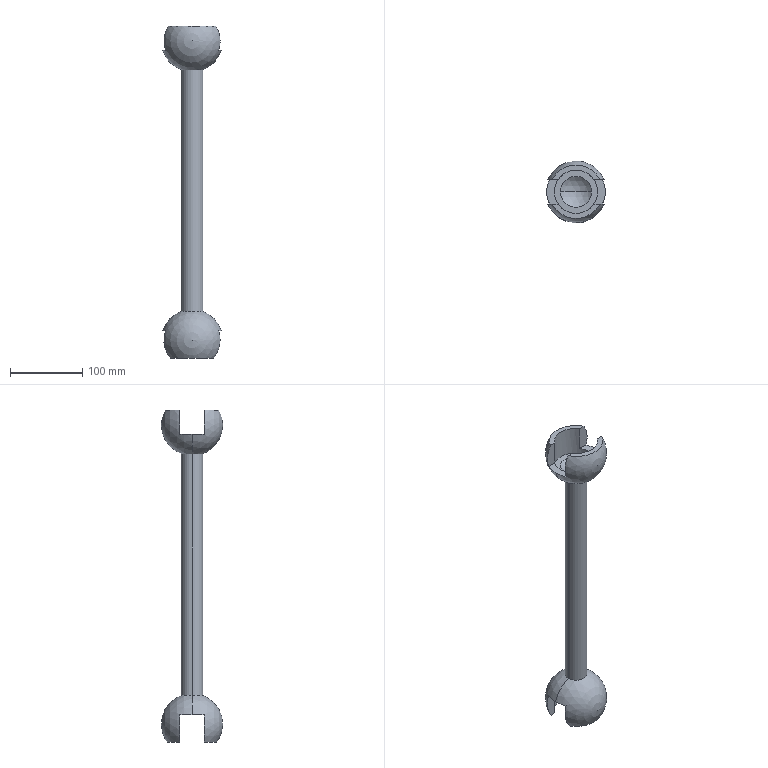Part | SolidWorks | features ICE 3, Chamfer 2, Extrusion 1, MirrorPattern 1, RevCut 1, Revolution 1 | 1 solid | 32 faces | box 80.921 x 85 x 459.451 mm | volume 470589 mm3 | plane 14 | sphere 8 | cylinder 6 | cone 4 | commonest cylinder face diameters 60 x4 30 x2
STEP:
#1=CARTESIAN_POINT('',(0.,0.,279.));
#2=VERTEX_POINT('',#1);
#3=CARTESIAN_POINT('',(-21.424,0.,288.));
#4=VERTEX_POINT('',#3);
#5=CARTESIAN_POINT('',(0.,0.,309.));
#6=DIRECTION('',(0.,1.,0.));
#7=DIRECTION('',(0.,0.,1.));
#8=AXIS2_PLACEMENT_3D('',#5,#6,#7);
#9=CIRCLE('',#8,30.);
#10=EDGE_CURVE('',#2,#4,#9,.T.);
#11=ORIENTED_EDGE('',*,*,#10,.F.);
#12=CARTESIAN_POINT('',(21.424,0.,288.));
#13=VERTEX_POINT('',#12);
#14=CARTESIAN_POINT('',(0.,0.,309.));
#15=DIRECTION('',(0.,-1.,0.));
#16=DIRECTION('',(1.,0.,0.));
#17=AXIS2_PLACEMENT_3D('',#14,#15,#16);
#18=CIRCLE('',#17,30.);
#19=EDGE_CURVE('',#2,#13,#18,.T.);
#20=ORIENTED_EDGE('',*,*,#19,.T.);
#21=CARTESIAN_POINT('',(0.,0.,288.));
#22=DIRECTION('',(0.,0.,1.));
#23=DIRECTION('',(-1.,0.,0.));
#24=AXIS2_PLACEMENT_3D('',#21,#22,#23);
#25=CIRCLE('',#24,21.424);
#26=EDGE_CURVE('',#13,#4,#25,.T.);
#27=ORIENTED_EDGE('',*,*,#26,.T.);
#28=EDGE_LOOP('',(#11,#20,#27));
#29=FACE_OUTER_BOUND('',#28,.T.);
#30=CARTESIAN_POINT('',(0.,0.,309.));
#31=DIRECTION('',(0.,-1.,0.));
#32=DIRECTION('',(-1.,0.,0.));
#33=AXIS2_PLACEMENT_3D('',#30,#31,#32);
#34=SPHERICAL_SURFACE('',#33,30.);
#35=ADVANCED_FACE('',(#29),#34,.F.);
#36=CARTESIAN_POINT('',(-30.,0.,288.));
#37=VERTEX_POINT('',#36);
#38=CARTESIAN_POINT('',(30.,0.,288.));
#39=VERTEX_POINT('',#38);
#40=CARTESIAN_POINT('',(0.,0.,288.));
#41=DIRECTION('',(0.,0.,1.));
#42=DIRECTION('',(1.,0.,0.));
#43=AXIS2_PLACEMENT_3D('',#40,#41,#42);
#44=CIRCLE('',#43,30.);
#45=EDGE_CURVE('',#37,#39,#44,.T.);
#46=ORIENTED_EDGE('',*,*,#45,.F.);
#47=CARTESIAN_POINT('',(-30.,0.,295.992));
#48=VERTEX_POINT('',#47);
#49=CARTESIAN_POINT('',(-30.,0.,288.));
#50=DIRECTION('',(0.,0.,1.));
#51=VECTOR('',#50,1000.);
#52=LINE('',#49,#51);
#53=EDGE_CURVE('',#37,#48,#52,.T.);
#54=ORIENTED_EDGE('',*,*,#53,.T.);
#55=CARTESIAN_POINT('',(-24.577,-17.204,295.992));
#56=VERTEX_POINT('',#55);
#57=CARTESIAN_POINT('',(0.,0.,295.992));
#58=DIRECTION('',(0.,0.,-1.));
#59=DIRECTION('',(1.,0.,0.));
#60=AXIS2_PLACEMENT_3D('',#57,#58,#59);
#61=CIRCLE('',#60,30.);
#62=EDGE_CURVE('',#56,#48,#61,.T.);
#63=ORIENTED_EDGE('',*,*,#62,.F.);
#64=CARTESIAN_POINT('',(-24.577,-17.204,329.749));
#65=VERTEX_POINT('',#64);
#66=CARTESIAN_POINT('',(-24.577,-17.204,288.));
#67=DIRECTION('',(0.,0.,1.));
#68=VECTOR('',#67,1000.);
#69=LINE('',#66,#68);
#70=EDGE_CURVE('',#56,#65,#69,.T.);
#71=ORIENTED_EDGE('',*,*,#70,.T.);
#72=CARTESIAN_POINT('',(24.577,-17.204,329.749));
#73=VERTEX_POINT('',#72);
#74=CARTESIAN_POINT('',(0.,0.,329.749));
#75=DIRECTION('',(0.,0.,1.));
#76=DIRECTION('',(-1.,0.,0.));
#77=AXIS2_PLACEMENT_3D('',#74,#75,#76);
#78=CIRCLE('',#77,30.);
#79=EDGE_CURVE('',#65,#73,#78,.T.);
#80=ORIENTED_EDGE('',*,*,#79,.T.);
#81=CARTESIAN_POINT('',(24.577,-17.204,295.992));
#82=VERTEX_POINT('',#81);
#83=CARTESIAN_POINT('',(24.577,-17.204,288.));
#84=DIRECTION('',(0.,0.,-1.));
#85=VECTOR('',#84,1000.);
#86=LINE('',#83,#85);
#87=EDGE_CURVE('',#73,#82,#86,.T.);
#88=ORIENTED_EDGE('',*,*,#87,.T.);
#89=CARTESIAN_POINT('',(30.,0.,295.992));
#90=VERTEX_POINT('',#89);
#91=CARTESIAN_POINT('',(0.,0.,295.992));
#92=DIRECTION('',(0.,0.,-1.));
#93=DIRECTION('',(1.,0.,0.));
#94=AXIS2_PLACEMENT_3D('',#91,#92,#93);
#95=CIRCLE('',#94,30.);
#96=EDGE_CURVE('',#90,#82,#95,.T.);
#97=ORIENTED_EDGE('',*,*,#96,.F.);
#98=CARTESIAN_POINT('',(30.,0.,288.));
#99=DIRECTION('',(0.,0.,1.));
#100=VECTOR('',#99,1000.);
#101=LINE('',#98,#100);
#102=EDGE_CURVE('',#39,#90,#101,.T.);
#103=ORIENTED_EDGE('',*,*,#102,.F.);
#104=EDGE_LOOP('',(#46,#54,#63,#71,#80,#88,#97,#103));
#105=FACE_OUTER_BOUND('',#104,.T.);
#106=CARTESIAN_POINT('',(0.,0.,288.));
#107=DIRECTION('',(0.,0.,1.));
#108=DIRECTION('',(1.,0.,0.));
#109=AXIS2_PLACEMENT_3D('',#106,#107,#108);
#110=CYLINDRICAL_SURFACE('',#109,30.);
#111=ADVANCED_FACE('',(#105),#110,.F.);
#112=CARTESIAN_POINT('',(15.,0.,269.235));
#113=VERTEX_POINT('',#112);
#114=CARTESIAN_POINT('',(-15.,0.,269.235));
#115=VERTEX_POINT('',#114);
#116=CARTESIAN_POINT('',(0.,0.,269.235));
#117=DIRECTION('',(0.,0.,1.));
#118=DIRECTION('',(1.,0.,0.));
#119=AXIS2_PLACEMENT_3D('',#116,#117,#118);
#120=CIRCLE('',#119,15.);
#121=EDGE_CURVE('',#113,#115,#120,.T.);
#122=ORIENTED_EDGE('',*,*,#121,.T.);
#123=CARTESIAN_POINT('',(-40.46,0.,295.992));
#124=VERTEX_POINT('',#123);
#125=CARTESIAN_POINT('',(0.,0.,309.));
#126=DIRECTION('',(0.,1.,0.));
#127=DIRECTION('',(-1.,0.,0.));
#128=AXIS2_PLACEMENT_3D('',#125,#126,#127);
#129=CIRCLE('',#128,42.5);
#130=EDGE_CURVE('',#115,#124,#129,.T.);
#131=ORIENTED_EDGE('',*,*,#130,.T.);
#132=CARTESIAN_POINT('',(-36.62,17.204,295.992));
#133=VERTEX_POINT('',#132);
#134=CARTESIAN_POINT('',(0.,0.,295.992));
#135=DIRECTION('',(0.,0.,1.));
#136=DIRECTION('',(1.,0.,0.));
#137=AXIS2_PLACEMENT_3D('',#134,#135,#136);
#138=CIRCLE('',#137,40.46);
#139=EDGE_CURVE('',#133,#124,#138,.T.);
#140=ORIENTED_EDGE('',*,*,#139,.F.);
#141=CARTESIAN_POINT('',(-32.854,17.204,329.757));
#142=VERTEX_POINT('',#141);
#143=CARTESIAN_POINT('',(0.,17.204,309.));
#144=DIRECTION('',(0.,-1.,0.));
#145=DIRECTION('',(0.,0.,-1.));
#146=AXIS2_PLACEMENT_3D('',#143,#144,#145);
#147=CIRCLE('',#146,38.862);
#148=EDGE_CURVE('',#142,#133,#147,.T.);
#149=ORIENTED_EDGE('',*,*,#148,.F.);
#150=CARTESIAN_POINT('',(32.854,17.204,329.757));
#151=VERTEX_POINT('',#150);
#152=CARTESIAN_POINT('',(0.,0.,329.757));
#153=DIRECTION('',(0.,0.,-1.));
#154=DIRECTION('',(-1.,0.,0.));
#155=AXIS2_PLACEMENT_3D('',#152,#153,#154);
#156=CIRCLE('',#155,37.086);
#157=EDGE_CURVE('',#142,#151,#156,.T.);
#158=ORIENTED_EDGE('',*,*,#157,.T.);
#159=CARTESIAN_POINT('',(36.62,17.204,295.992));
#160=VERTEX_POINT('',#159);
#161=CARTESIAN_POINT('',(0.,17.204,309.));
#162=DIRECTION('',(0.,-1.,0.));
#163=DIRECTION('',(0.,0.,-1.));
#164=AXIS2_PLACEMENT_3D('',#161,#162,#163);
#165=CIRCLE('',#164,38.862);
#166=EDGE_CURVE('',#160,#151,#165,.T.);
#167=ORIENTED_EDGE('',*,*,#166,.F.);
#168=CARTESIAN_POINT('',(40.46,0.,295.992));
#169=VERTEX_POINT('',#168);
#170=CARTESIAN_POINT('',(0.,0.,295.992));
#171=DIRECTION('',(0.,0.,1.));
#172=DIRECTION('',(1.,0.,0.));
#173=AXIS2_PLACEMENT_3D('',#170,#171,#172);
#174=CIRCLE('',#173,40.46);
#175=EDGE_CURVE('',#169,#160,#174,.T.);
#176=ORIENTED_EDGE('',*,*,#175,.F.);
#177=CARTESIAN_POINT('',(0.,0.,309.));
#178=DIRECTION('',(0.,-1.,0.));
#179=DIRECTION('',(0.,0.,-1.));
#180=AXIS2_PLACEMENT_3D('',#177,#178,#179);
#181=CIRCLE('',#180,42.5);
#182=EDGE_CURVE('',#113,#169,#181,.T.);
#183=ORIENTED_EDGE('',*,*,#182,.F.);
#184=EDGE_LOOP('',(#122,#131,#140,#149,#158,#167,#176,#183));
#185=FACE_OUTER_BOUND('',#184,.T.);
#186=CARTESIAN_POINT('',(0.,0.,309.));
#187=DIRECTION('',(0.,1.,0.));
#188=DIRECTION('',(1.,0.,0.));
#189=AXIS2_PLACEMENT_3D('',#186,#187,#188);
#190=SPHERICAL_SURFACE('',#189,42.5);
#191=ADVANCED_FACE('',(#185),#190,.T.);
#192=CARTESIAN_POINT('',(0.,0.,-75.));
#193=VERTEX_POINT('',#192);
#194=CARTESIAN_POINT('',(-21.424,0.,-84.));
#195=VERTEX_POINT('',#194);
#196=CARTESIAN_POINT('',(0.,0.,-105.));
#197=DIRECTION('',(0.,-1.,0.));
#198=DIRECTION('',(0.,0.,-1.));
#199=AXIS2_PLACEMENT_3D('',#196,#197,#198);
#200=CIRCLE('',#199,30.);
#201=EDGE_CURVE('',#193,#195,#200,.T.);
#202=ORIENTED_EDGE('',*,*,#201,.F.);
#203=CARTESIAN_POINT('',(21.424,0.,-84.));
#204=VERTEX_POINT('',#203);
#205=CARTESIAN_POINT('',(0.,0.,-105.));
#206=DIRECTION('',(0.,1.,0.));
#207=DIRECTION('',(-1.,0.,0.));
#208=AXIS2_PLACEMENT_3D('',#205,#206,#207);
#209=CIRCLE('',#208,30.);
#210=EDGE_CURVE('',#193,#204,#209,.T.);
#211=ORIENTED_EDGE('',*,*,#210,.T.);
#212=CARTESIAN_POINT('',(0.,0.,-84.));
#213=DIRECTION('',(0.,0.,-1.));
#214=DIRECTION('',(1.,0.,0.));
#215=AXIS2_PLACEMENT_3D('',#212,#213,#214);
#216=CIRCLE('',#215,21.424);
#217=EDGE_CURVE('',#204,#195,#216,.T.);
#218=ORIENTED_EDGE('',*,*,#217,.T.);
#219=EDGE_LOOP('',(#202,#211,#218));
#220=FACE_OUTER_BOUND('',#219,.T.);
#221=CARTESIAN_POINT('',(0.,0.,-105.));
#222=DIRECTION('',(0.,1.,0.));
#223=DIRECTION('',(-1.,0.,0.));
#224=AXIS2_PLACEMENT_3D('',#221,#222,#223);
#225=SPHERICAL_SURFACE('',#224,30.);
#226=ADVANCED_FACE('',(#220),#225,.F.);
#227=CARTESIAN_POINT('',(15.,0.,-65.235));
#228=VERTEX_POINT('',#227);
#229=CARTESIAN_POINT('',(-15.,0.,-65.235));
#230=VERTEX_POINT('',#229);
#231=CARTESIAN_POINT('',(0.,0.,-65.235));
#232=DIRECTION('',(0.,0.,-1.));
#233=DIRECTION('',(-1.,0.,0.));
#234=AXIS2_PLACEMENT_3D('',#231,#232,#233);
#235=CIRCLE('',#234,15.);
#236=EDGE_CURVE('',#228,#230,#235,.T.);
#237=ORIENTED_EDGE('',*,*,#236,.T.);
#238=CARTESIAN_POINT('',(-40.46,0.,-91.992));
#239=VERTEX_POINT('',#238);
#240=CARTESIAN_POINT('',(0.,0.,-105.));
#241=DIRECTION('',(0.,-1.,0.));
#242=DIRECTION('',(1.,0.,0.));
#243=AXIS2_PLACEMENT_3D('',#240,#241,#242);
#244=CIRCLE('',#243,42.5);
#245=EDGE_CURVE('',#230,#239,#244,.T.);
#246=ORIENTED_EDGE('',*,*,#245,.T.);
#247=CARTESIAN_POINT('',(-36.62,-17.204,-91.992));
#248=VERTEX_POINT('',#247);
#249=CARTESIAN_POINT('',(0.,0.,-91.992));
#250=DIRECTION('',(0.,0.,1.));
#251=DIRECTION('',(1.,0.,0.));
#252=AXIS2_PLACEMENT_3D('',#249,#250,#251);
#253=CIRCLE('',#252,40.46);
#254=EDGE_CURVE('',#239,#248,#253,.T.);
#255=ORIENTED_EDGE('',*,*,#254,.T.);
#256=CARTESIAN_POINT('',(-30.008,-17.204,-129.694));
#257=VERTEX_POINT('',#256);
#258=CARTESIAN_POINT('',(0.,-17.204,-105.));
#259=DIRECTION('',(0.,1.,0.));
#260=DIRECTION('',(0.,0.,1.));
#261=AXIS2_PLACEMENT_3D('',#258,#259,#260);
#262=CIRCLE('',#261,38.862);
#263=EDGE_CURVE('',#257,#248,#262,.T.);
#264=ORIENTED_EDGE('',*,*,#263,.F.);
#265=CARTESIAN_POINT('',(30.008,-17.204,-129.694));
#266=VERTEX_POINT('',#265);
#267=CARTESIAN_POINT('',(0.,0.,-129.694));
#268=DIRECTION('',(0.,0.,1.));
#269=DIRECTION('',(1.,0.,0.));
#270=AXIS2_PLACEMENT_3D('',#267,#268,#269);
#271=CIRCLE('',#270,34.59);
#272=EDGE_CURVE('',#257,#266,#271,.T.);
#273=ORIENTED_EDGE('',*,*,#272,.T.);
#274=CARTESIAN_POINT('',(36.62,-17.204,-91.992));
#275=VERTEX_POINT('',#274);
#276=CARTESIAN_POINT('',(0.,-17.204,-105.));
#277=DIRECTION('',(0.,1.,0.));
#278=DIRECTION('',(0.,0.,1.));
#279=AXIS2_PLACEMENT_3D('',#276,#277,#278);
#280=CIRCLE('',#279,38.862);
#281=EDGE_CURVE('',#275,#266,#280,.T.);
#282=ORIENTED_EDGE('',*,*,#281,.F.);
#283=CARTESIAN_POINT('',(40.46,0.,-91.992));
#284=VERTEX_POINT('',#283);
#285=CARTESIAN_POINT('',(0.,0.,-91.992));
#286=DIRECTION('',(0.,0.,1.));
#287=DIRECTION('',(1.,0.,0.));
#288=AXIS2_PLACEMENT_3D('',#285,#286,#287);
#289=CIRCLE('',#288,40.46);
#290=EDGE_CURVE('',#275,#284,#289,.T.);
#291=ORIENTED_EDGE('',*,*,#290,.T.);
#292=CARTESIAN_POINT('',(0.,0.,-105.));
#293=DIRECTION('',(0.,1.,0.));
#294=DIRECTION('',(0.,0.,1.));
#295=AXIS2_PLACEMENT_3D('',#292,#293,#294);
#296=CIRCLE('',#295,42.5);
#297=EDGE_CURVE('',#228,#284,#296,.T.);
#298=ORIENTED_EDGE('',*,*,#297,.F.);
#299=EDGE_LOOP('',(#237,#246,#255,#264,#273,#282,#291,#298));
#300=FACE_OUTER_BOUND('',#299,.T.);
#301=CARTESIAN_POINT('',(0.,0.,-105.));
#302=DIRECTION('',(0.,-1.,0.));
#303=DIRECTION('',(1.,0.,0.));
#304=AXIS2_PLACEMENT_3D('',#301,#302,#303);
#305=SPHERICAL_SURFACE('',#304,42.5);
#306=ADVANCED_FACE('',(#300),#305,.T.);
#307=CARTESIAN_POINT('',(-30.,0.,-84.));
#308=VERTEX_POINT('',#307);
#309=CARTESIAN_POINT('',(30.,0.,-84.));
#310=VERTEX_POINT('',#309);
#311=CARTESIAN_POINT('',(0.,0.,-84.));
#312=DIRECTION('',(0.,0.,1.));
#313=DIRECTION('',(1.,0.,0.));
#314=AXIS2_PLACEMENT_3D('',#311,#312,#313);
#315=CIRCLE('',#314,30.);
#316=EDGE_CURVE('',#308,#310,#315,.T.);
#317=ORIENTED_EDGE('',*,*,#316,.T.);
#318=CARTESIAN_POINT('',(30.,0.,-91.992));
#319=VERTEX_POINT('',#318);
#320=CARTESIAN_POINT('',(30.,0.,-84.));
#321=DIRECTION('',(0.,0.,-1.));
#322=VECTOR('',#321,1000.);
#323=LINE('',#320,#322);
#324=EDGE_CURVE('',#310,#319,#323,.T.);
#325=ORIENTED_EDGE('',*,*,#324,.T.);
#326=CARTESIAN_POINT('',(24.577,-17.204,-91.992));
#327=VERTEX_POINT('',#326);
#328=CARTESIAN_POINT('',(0.,0.,-91.992));
#329=DIRECTION('',(0.,0.,1.));
#330=DIRECTION('',(1.,0.,0.));
#331=AXIS2_PLACEMENT_3D('',#328,#329,#330);
#332=CIRCLE('',#331,30.);
#333=EDGE_CURVE('',#327,#319,#332,.T.);
#334=ORIENTED_EDGE('',*,*,#333,.F.);
#335=CARTESIAN_POINT('',(24.577,-17.204,-125.104));
#336=VERTEX_POINT('',#335);
#337=CARTESIAN_POINT('',(24.577,-17.204,-84.));
#338=DIRECTION('',(0.,0.,-1.));
#339=VECTOR('',#338,1000.);
#340=LINE('',#337,#339);
#341=EDGE_CURVE('',#327,#336,#340,.T.);
#342=ORIENTED_EDGE('',*,*,#341,.T.);
#343=CARTESIAN_POINT('',(-24.577,-17.204,-125.104));
#344=VERTEX_POINT('',#343);
#345=CARTESIAN_POINT('',(0.,0.,-125.104));
#346=DIRECTION('',(0.,0.,-1.));
#347=DIRECTION('',(1.,0.,0.));
#348=AXIS2_PLACEMENT_3D('',#345,#346,#347);
#349=CIRCLE('',#348,30.);
#350=EDGE_CURVE('',#336,#344,#349,.T.);
#351=ORIENTED_EDGE('',*,*,#350,.T.);
#352=CARTESIAN_POINT('',(-24.577,-17.204,-91.992));
#353=VERTEX_POINT('',#352);
#354=CARTESIAN_POINT('',(-24.577,-17.204,-84.));
#355=DIRECTION('',(0.,0.,1.));
#356=VECTOR('',#355,1000.);
#357=LINE('',#354,#356);
#358=EDGE_CURVE('',#344,#353,#357,.T.);
#359=ORIENTED_EDGE('',*,*,#358,.T.);
#360=CARTESIAN_POINT('',(-30.,0.,-91.992));
#361=VERTEX_POINT('',#360);
#362=CARTESIAN_POINT('',(0.,0.,-91.992));
#363=DIRECTION('',(0.,0.,1.));
#364=DIRECTION('',(1.,0.,0.));
#365=AXIS2_PLACEMENT_3D('',#362,#363,#364);
#366=CIRCLE('',#365,30.);
#367=EDGE_CURVE('',#361,#353,#366,.T.);
#368=ORIENTED_EDGE('',*,*,#367,.F.);
#369=CARTESIAN_POINT('',(-30.,0.,-84.));
#370=DIRECTION('',(0.,0.,-1.));
#371=VECTOR('',#370,1000.);
#372=LINE('',#369,#371);
#373=EDGE_CURVE('',#308,#361,#372,.T.);
#374=ORIENTED_EDGE('',*,*,#373,.F.);
#375=EDGE_LOOP('',(#317,#325,#334,#342,#351,#359,#368,#374));
#376=FACE_OUTER_BOUND('',#375,.T.);
#377=CARTESIAN_POINT('',(0.,0.,-84.));
#378=DIRECTION('',(0.,0.,-1.));
#379=DIRECTION('',(-1.,0.,0.));
#380=AXIS2_PLACEMENT_3D('',#377,#378,#379);
#381=CYLINDRICAL_SURFACE('',#380,30.);
#382=ADVANCED_FACE('',(#376),#381,.F.);
#383=ORIENTED_EDGE('',*,*,#121,.F.);
#384=CARTESIAN_POINT('',(15.,0.,80.));
#385=DIRECTION('',(0.,0.,-1.));
#386=VECTOR('',#385,1000.);
#387=LINE('',#384,#386);
#388=EDGE_CURVE('',#113,#228,#387,.T.);
#389=ORIENTED_EDGE('',*,*,#388,.T.);
#390=CARTESIAN_POINT('',(0.,0.,-65.235));
#391=DIRECTION('',(0.,0.,-1.));
#392=DIRECTION('',(-1.,0.,0.));
#393=AXIS2_PLACEMENT_3D('',#390,#391,#392);
#394=CIRCLE('',#393,15.);
#395=EDGE_CURVE('',#230,#228,#394,.T.);
#396=ORIENTED_EDGE('',*,*,#395,.F.);
#397=CARTESIAN_POINT('',(-15.,0.,80.));
#398=DIRECTION('',(0.,0.,-1.));
#399=VECTOR('',#398,1000.);
#400=LINE('',#397,#399);
#401=EDGE_CURVE('',#115,#230,#400,.T.);
#402=ORIENTED_EDGE('',*,*,#401,.F.);
#403=EDGE_LOOP('',(#383,#389,#396,#402));
#404=FACE_OUTER_BOUND('',#403,.T.);
#405=CARTESIAN_POINT('',(0.,0.,80.));
#406=DIRECTION('',(0.,0.,-1.));
#407=DIRECTION('',(-1.,0.,0.));
#408=AXIS2_PLACEMENT_3D('',#405,#406,#407);
#409=CYLINDRICAL_SURFACE('',#408,15.);
#410=ADVANCED_FACE('',(#404),#409,.T.);
#411=ORIENTED_EDGE('',*,*,#388,.F.);
#412=CARTESIAN_POINT('',(0.,0.,269.235));
#413=DIRECTION('',(0.,0.,1.));
#414=DIRECTION('',(1.,0.,0.));
#415=AXIS2_PLACEMENT_3D('',#412,#413,#414);
#416=CIRCLE('',#415,15.);
#417=EDGE_CURVE('',#115,#113,#416,.T.);
#418=ORIENTED_EDGE('',*,*,#417,.F.);
#419=ORIENTED_EDGE('',*,*,#401,.T.);
#420=ORIENTED_EDGE('',*,*,#236,.F.);
#421=EDGE_LOOP('',(#411,#418,#419,#420));
#422=FACE_OUTER_BOUND('',#421,.T.);
#423=CARTESIAN_POINT('',(0.,0.,80.));
#424=DIRECTION('',(0.,0.,-1.));
#425=DIRECTION('',(-1.,0.,0.));
#426=AXIS2_PLACEMENT_3D('',#423,#424,#425);
#427=CYLINDRICAL_SURFACE('',#426,15.);
#428=ADVANCED_FACE('',(#422),#427,.T.);
#429=ORIENTED_EDGE('',*,*,#324,.F.);
#430=CARTESIAN_POINT('',(0.,0.,-84.));
#431=DIRECTION('',(0.,0.,1.));
#432=DIRECTION('',(1.,0.,0.));
#433=AXIS2_PLACEMENT_3D('',#430,#431,#432);
#434=CIRCLE('',#433,30.);
#435=EDGE_CURVE('',#310,#308,#434,.T.);
#436=ORIENTED_EDGE('',*,*,#435,.T.);
#437=ORIENTED_EDGE('',*,*,#373,.T.);
#438=CARTESIAN_POINT('',(-24.577,17.204,-91.992));
#439=VERTEX_POINT('',#438);
#440=CARTESIAN_POINT('',(0.,0.,-91.992));
#441=DIRECTION('',(0.,0.,1.));
#442=DIRECTION('',(1.,0.,0.));
#443=AXIS2_PLACEMENT_3D('',#440,#441,#442);
#444=CIRCLE('',#443,30.);
#445=EDGE_CURVE('',#439,#361,#444,.T.);
#446=ORIENTED_EDGE('',*,*,#445,.F.);
#447=CARTESIAN_POINT('',(-24.577,17.204,-125.104));
#448=VERTEX_POINT('',#447);
#449=CARTESIAN_POINT('',(-24.577,17.204,-84.));
#450=DIRECTION('',(0.,0.,1.));
#451=VECTOR('',#450,1000.);
#452=LINE('',#449,#451);
#453=EDGE_CURVE('',#448,#439,#452,.T.);
#454=ORIENTED_EDGE('',*,*,#453,.F.);
#455=CARTESIAN_POINT('',(24.577,17.204,-125.104));
#456=VERTEX_POINT('',#455);
#457=CARTESIAN_POINT('',(0.,0.,-125.104));
#458=DIRECTION('',(0.,0.,-1.));
#459=DIRECTION('',(1.,0.,0.));
#460=AXIS2_PLACEMENT_3D('',#457,#458,#459);
#461=CIRCLE('',#460,30.);
#462=EDGE_CURVE('',#448,#456,#461,.T.);
#463=ORIENTED_EDGE('',*,*,#462,.T.);
#464=CARTESIAN_POINT('',(24.577,17.204,-91.992));
#465=VERTEX_POINT('',#464);
#466=CARTESIAN_POINT('',(24.577,17.204,-84.));
#467=DIRECTION('',(0.,0.,-1.));
#468=VECTOR('',#467,1000.);
#469=LINE('',#466,#468);
#470=EDGE_CURVE('',#465,#456,#469,.T.);
#471=ORIENTED_EDGE('',*,*,#470,.F.);
#472=CARTESIAN_POINT('',(0.,0.,-91.992));
#473=DIRECTION('',(0.,0.,1.));
#474=DIRECTION('',(1.,0.,0.));
#475=AXIS2_PLACEMENT_3D('',#472,#473,#474);
#476=CIRCLE('',#475,30.);
#477=EDGE_CURVE('',#319,#465,#476,.T.);
#478=ORIENTED_EDGE('',*,*,#477,.F.);
#479=EDGE_LOOP('',(#429,#436,#437,#446,#454,#463,#471,#478));
#480=FACE_OUTER_BOUND('',#479,.T.);
#481=CARTESIAN_POINT('',(0.,0.,-84.));
#482=DIRECTION('',(0.,0.,-1.));
#483=DIRECTION('',(-1.,0.,0.));
#484=AXIS2_PLACEMENT_3D('',#481,#482,#483);
#485=CYLINDRICAL_SURFACE('',#484,30.);
#486=ADVANCED_FACE('',(#480),#485,.F.);
#487=ORIENTED_EDGE('',*,*,#245,.F.);
#488=ORIENTED_EDGE('',*,*,#395,.T.);
#489=ORIENTED_EDGE('',*,*,#297,.T.);
#490=CARTESIAN_POINT('',(36.62,17.204,-91.992));
#491=VERTEX_POINT('',#490);
#492=CARTESIAN_POINT('',(0.,0.,-91.992));
#493=DIRECTION('',(0.,0.,1.));
#494=DIRECTION('',(1.,0.,0.));
#495=AXIS2_PLACEMENT_3D('',#492,#493,#494);
#496=CIRCLE('',#495,40.46);
#497=EDGE_CURVE('',#284,#491,#496,.T.);
#498=ORIENTED_EDGE('',*,*,#497,.T.);
#499=CARTESIAN_POINT('',(30.008,17.204,-129.694));
#500=VERTEX_POINT('',#499);
#501=CARTESIAN_POINT('',(0.,17.204,-105.));
#502=DIRECTION('',(0.,1.,0.));
#503=DIRECTION('',(0.,0.,1.));
#504=AXIS2_PLACEMENT_3D('',#501,#502,#503);
#505=CIRCLE('',#504,38.862);
#506=EDGE_CURVE('',#491,#500,#505,.T.);
#507=ORIENTED_EDGE('',*,*,#506,.T.);
#508=CARTESIAN_POINT('',(-30.008,17.204,-129.694));
#509=VERTEX_POINT('',#508);
#510=CARTESIAN_POINT('',(0.,0.,-129.694));
#511=DIRECTION('',(0.,0.,1.));
#512=DIRECTION('',(1.,0.,0.));
#513=AXIS2_PLACEMENT_3D('',#510,#511,#512);
#514=CIRCLE('',#513,34.59);
#515=EDGE_CURVE('',#500,#509,#514,.T.);
#516=ORIENTED_EDGE('',*,*,#515,.T.);
#517=CARTESIAN_POINT('',(-36.62,17.204,-91.992));
#518=VERTEX_POINT('',#517);
#519=CARTESIAN_POINT('',(0.,17.204,-105.));
#520=DIRECTION('',(0.,1.,0.));
#521=DIRECTION('',(0.,0.,1.));
#522=AXIS2_PLACEMENT_3D('',#519,#520,#521);
#523=CIRCLE('',#522,38.862);
#524=EDGE_CURVE('',#509,#518,#523,.T.);
#525=ORIENTED_EDGE('',*,*,#524,.T.);
#526=CARTESIAN_POINT('',(0.,0.,-91.992));
#527=DIRECTION('',(0.,0.,1.));
#528=DIRECTION('',(1.,0.,0.));
#529=AXIS2_PLACEMENT_3D('',#526,#527,#528);
#530=CIRCLE('',#529,40.46);
#531=EDGE_CURVE('',#518,#239,#530,.T.);
#532=ORIENTED_EDGE('',*,*,#531,.T.);
#533=EDGE_LOOP('',(#487,#488,#489,#498,#507,#516,#525,#532));
#534=FACE_OUTER_BOUND('',#533,.T.);
#535=CARTESIAN_POINT('',(0.,0.,-105.));
#536=DIRECTION('',(0.,-1.,0.));
#537=DIRECTION('',(1.,0.,0.));
#538=AXIS2_PLACEMENT_3D('',#535,#536,#537);
#539=SPHERICAL_SURFACE('',#538,42.5);
#540=ADVANCED_FACE('',(#534),#539,.T.);
#541=ORIENTED_EDGE('',*,*,#210,.F.);
#542=ORIENTED_EDGE('',*,*,#201,.T.);
#543=CARTESIAN_POINT('',(0.,0.,-84.));
#544=DIRECTION('',(0.,0.,-1.));
#545=DIRECTION('',(1.,0.,0.));
#546=AXIS2_PLACEMENT_3D('',#543,#544,#545);
#547=CIRCLE('',#546,21.424);
#548=EDGE_CURVE('',#195,#204,#547,.T.);
#549=ORIENTED_EDGE('',*,*,#548,.T.);
#550=EDGE_LOOP('',(#541,#542,#549));
#551=FACE_OUTER_BOUND('',#550,.T.);
#552=CARTESIAN_POINT('',(0.,0.,-105.));
#553=DIRECTION('',(0.,1.,0.));
#554=DIRECTION('',(-1.,0.,0.));
#555=AXIS2_PLACEMENT_3D('',#552,#553,#554);
#556=SPHERICAL_SURFACE('',#555,30.);
#557=ADVANCED_FACE('',(#551),#556,.F.);
#558=ORIENTED_EDGE('',*,*,#316,.F.);
#559=ORIENTED_EDGE('',*,*,#435,.F.);
#560=EDGE_LOOP('',(#558,#559));
#561=FACE_OUTER_BOUND('',#560,.T.);
#562=ORIENTED_EDGE('',*,*,#548,.F.);
#563=ORIENTED_EDGE('',*,*,#217,.F.);
#564=EDGE_LOOP('',(#562,#563));
#565=FACE_BOUND('',#564,.T.);
#566=CARTESIAN_POINT('',(0.,0.,-84.));
#567=DIRECTION('',(0.,0.,1.));
#568=DIRECTION('',(1.,0.,0.));
#569=AXIS2_PLACEMENT_3D('',#566,#567,#568);
#570=PLANE('',#569);
#571=ADVANCED_FACE('',(#561,#565),#570,.F.);
#572=ORIENTED_EDGE('',*,*,#524,.F.);
#573=CARTESIAN_POINT('',(-30.008,17.204,-129.694));
#574=CARTESIAN_POINT('',(-28.217,17.204,-128.14));
#575=CARTESIAN_POINT('',(-26.411,17.204,-126.606));
#576=CARTESIAN_POINT('',(-24.577,17.204,-125.104));
#577=B_SPLINE_CURVE_WITH_KNOTS('',3,(#573,#574,#575,#576),.UNSPECIFIED.,.F.,.F.,(4,4),(0.,0.007111),.UNSPECIFIED.);
#578=EDGE_CURVE('',#509,#448,#577,.T.);
#579=ORIENTED_EDGE('',*,*,#578,.T.);
#580=ORIENTED_EDGE('',*,*,#453,.T.);
#581=CARTESIAN_POINT('',(-75.5,17.204,-91.992));
#582=DIRECTION('',(1.,0.,0.));
#583=VECTOR('',#582,1000.);
#584=LINE('',#581,#583);
#585=EDGE_CURVE('',#518,#439,#584,.T.);
#586=ORIENTED_EDGE('',*,*,#585,.F.);
#587=EDGE_LOOP('',(#572,#579,#580,#586));
#588=FACE_OUTER_BOUND('',#587,.T.);
#589=CARTESIAN_POINT('',(-75.5,17.204,-178.216));
#590=DIRECTION('',(0.,1.,0.));
#591=DIRECTION('',(0.,0.,1.));
#592=AXIS2_PLACEMENT_3D('',#589,#590,#591);
#593=PLANE('',#592);
#594=ADVANCED_FACE('',(#588),#593,.F.);
#595=ORIENTED_EDGE('',*,*,#445,.T.);
#596=ORIENTED_EDGE('',*,*,#367,.T.);
#597=CARTESIAN_POINT('',(-75.5,-17.204,-91.992));
#598=DIRECTION('',(1.,0.,0.));
#599=VECTOR('',#598,1000.);
#600=LINE('',#597,#599);
#601=EDGE_CURVE('',#248,#353,#600,.T.);
#602=ORIENTED_EDGE('',*,*,#601,.F.);
#603=ORIENTED_EDGE('',*,*,#254,.F.);
#604=ORIENTED_EDGE('',*,*,#531,.F.);
#605=ORIENTED_EDGE('',*,*,#585,.T.);
#606=EDGE_LOOP('',(#595,#596,#602,#603,#604,#605));
#607=FACE_OUTER_BOUND('',#606,.T.);
#608=CARTESIAN_POINT('',(-75.5,17.204,-91.992));
#609=DIRECTION('',(0.,0.,1.));
#610=DIRECTION('',(1.,0.,0.));
#611=AXIS2_PLACEMENT_3D('',#608,#609,#610);
#612=PLANE('',#611);
#613=ADVANCED_FACE('',(#607),#612,.F.);
#614=ORIENTED_EDGE('',*,*,#358,.F.);
#615=CARTESIAN_POINT('',(-24.577,-17.204,-125.104));
#616=CARTESIAN_POINT('',(-26.411,-17.204,-126.606));
#617=CARTESIAN_POINT('',(-28.217,-17.204,-128.14));
#618=CARTESIAN_POINT('',(-30.008,-17.204,-129.694));
#619=B_SPLINE_CURVE_WITH_KNOTS('',3,(#615,#616,#617,#618),.UNSPECIFIED.,.F.,.F.,(4,4),(0.,0.007111),.UNSPECIFIED.);
#620=EDGE_CURVE('',#344,#257,#619,.T.);
#621=ORIENTED_EDGE('',*,*,#620,.T.);
#622=ORIENTED_EDGE('',*,*,#263,.T.);
#623=ORIENTED_EDGE('',*,*,#601,.T.);
#624=EDGE_LOOP('',(#614,#621,#622,#623));
#625=FACE_OUTER_BOUND('',#624,.T.);
#626=CARTESIAN_POINT('',(-75.5,-17.204,-178.216));
#627=DIRECTION('',(0.,1.,0.));
#628=DIRECTION('',(0.,0.,1.));
#629=AXIS2_PLACEMENT_3D('',#626,#627,#628);
#630=PLANE('',#629);
#631=ADVANCED_FACE('',(#625),#630,.T.);
#632=ORIENTED_EDGE('',*,*,#281,.T.);
#633=CARTESIAN_POINT('',(30.008,-17.204,-129.694));
#634=CARTESIAN_POINT('',(28.217,-17.204,-128.14));
#635=CARTESIAN_POINT('',(26.411,-17.204,-126.606));
#636=CARTESIAN_POINT('',(24.577,-17.204,-125.104));
#637=B_SPLINE_CURVE_WITH_KNOTS('',3,(#633,#634,#635,#636),.UNSPECIFIED.,.F.,.F.,(4,4),(0.,0.007111),.UNSPECIFIED.);
#638=EDGE_CURVE('',#266,#336,#637,.T.);
#639=ORIENTED_EDGE('',*,*,#638,.T.);
#640=ORIENTED_EDGE('',*,*,#341,.F.);
#641=CARTESIAN_POINT('',(-75.5,-17.204,-91.992));
#642=DIRECTION('',(1.,0.,0.));
#643=VECTOR('',#642,1000.);
#644=LINE('',#641,#643);
#645=EDGE_CURVE('',#327,#275,#644,.T.);
#646=ORIENTED_EDGE('',*,*,#645,.T.);
#647=EDGE_LOOP('',(#632,#639,#640,#646));
#648=FACE_OUTER_BOUND('',#647,.T.);
#649=CARTESIAN_POINT('',(-75.5,-17.204,-178.216));
#650=DIRECTION('',(0.,1.,0.));
#651=DIRECTION('',(0.,0.,1.));
#652=AXIS2_PLACEMENT_3D('',#649,#650,#651);
#653=PLANE('',#652);
#654=ADVANCED_FACE('',(#648),#653,.T.);
#655=ORIENTED_EDGE('',*,*,#333,.T.);
#656=ORIENTED_EDGE('',*,*,#477,.T.);
#657=CARTESIAN_POINT('',(-75.5,17.204,-91.992));
#658=DIRECTION('',(1.,0.,0.));
#659=VECTOR('',#658,1000.);
#660=LINE('',#657,#659);
#661=EDGE_CURVE('',#465,#491,#660,.T.);
#662=ORIENTED_EDGE('',*,*,#661,.T.);
#663=ORIENTED_EDGE('',*,*,#497,.F.);
#664=ORIENTED_EDGE('',*,*,#290,.F.);
#665=ORIENTED_EDGE('',*,*,#645,.F.);
#666=EDGE_LOOP('',(#655,#656,#662,#663,#664,#665));
#667=FACE_OUTER_BOUND('',#666,.T.);
#668=CARTESIAN_POINT('',(-75.5,17.204,-91.992));
#669=DIRECTION('',(0.,0.,1.));
#670=DIRECTION('',(1.,0.,0.));
#671=AXIS2_PLACEMENT_3D('',#668,#669,#670);
#672=PLANE('',#671);
#673=ADVANCED_FACE('',(#667),#672,.F.);
#674=ORIENTED_EDGE('',*,*,#470,.T.);
#675=CARTESIAN_POINT('',(24.577,17.204,-125.104));
#676=CARTESIAN_POINT('',(26.411,17.204,-126.606));
#677=CARTESIAN_POINT('',(28.217,17.204,-128.14));
#678=CARTESIAN_POINT('',(30.008,17.204,-129.694));
#679=B_SPLINE_CURVE_WITH_KNOTS('',3,(#675,#676,#677,#678),.UNSPECIFIED.,.F.,.F.,(4,4),(0.,0.007111),.UNSPECIFIED.);
#680=EDGE_CURVE('',#456,#500,#679,.T.);
#681=ORIENTED_EDGE('',*,*,#680,.T.);
#682=ORIENTED_EDGE('',*,*,#506,.F.);
#683=ORIENTED_EDGE('',*,*,#661,.F.);
#684=EDGE_LOOP('',(#674,#681,#682,#683));
#685=FACE_OUTER_BOUND('',#684,.T.);
#686=CARTESIAN_POINT('',(-75.5,17.204,-178.216));
#687=DIRECTION('',(0.,1.,0.));
#688=DIRECTION('',(0.,0.,1.));
#689=AXIS2_PLACEMENT_3D('',#686,#687,#688);
#690=PLANE('',#689);
#691=ADVANCED_FACE('',(#685),#690,.F.);
#692=ORIENTED_EDGE('',*,*,#638,.F.);
#693=ORIENTED_EDGE('',*,*,#272,.F.);
#694=ORIENTED_EDGE('',*,*,#620,.F.);
#695=ORIENTED_EDGE('',*,*,#350,.F.);
#696=EDGE_LOOP('',(#692,#693,#694,#695));
#697=FACE_OUTER_BOUND('',#696,.T.);
#698=CARTESIAN_POINT('',(0.,0.,-125.104));
#699=DIRECTION('',(0.,0.,-1.));
#700=DIRECTION('',(-1.,0.,0.));
#701=AXIS2_PLACEMENT_3D('',#698,#699,#700);
#702=CONICAL_SURFACE('',#701,30.,0.7854);
#703=ADVANCED_FACE('',(#697),#702,.F.);
#704=ORIENTED_EDGE('',*,*,#578,.F.);
#705=ORIENTED_EDGE('',*,*,#515,.F.);
#706=ORIENTED_EDGE('',*,*,#680,.F.);
#707=ORIENTED_EDGE('',*,*,#462,.F.);
#708=EDGE_LOOP('',(#704,#705,#706,#707));
#709=FACE_OUTER_BOUND('',#708,.T.);
#710=CARTESIAN_POINT('',(0.,0.,-125.104));
#711=DIRECTION('',(0.,0.,-1.));
#712=DIRECTION('',(-1.,0.,0.));
#713=AXIS2_PLACEMENT_3D('',#710,#711,#712);
#714=CONICAL_SURFACE('',#713,30.,0.7854);
#715=ADVANCED_FACE('',(#709),#714,.F.);
#716=ORIENTED_EDGE('',*,*,#130,.F.);
#717=ORIENTED_EDGE('',*,*,#417,.T.);
#718=ORIENTED_EDGE('',*,*,#182,.T.);
#719=CARTESIAN_POINT('',(36.62,-17.204,295.992));
#720=VERTEX_POINT('',#719);
#721=CARTESIAN_POINT('',(0.,0.,295.992));
#722=DIRECTION('',(0.,0.,1.));
#723=DIRECTION('',(1.,0.,0.));
#724=AXIS2_PLACEMENT_3D('',#721,#722,#723);
#725=CIRCLE('',#724,40.46);
#726=EDGE_CURVE('',#720,#169,#725,.T.);
#727=ORIENTED_EDGE('',*,*,#726,.F.);
#728=CARTESIAN_POINT('',(32.854,-17.204,329.757));
#729=VERTEX_POINT('',#728);
#730=CARTESIAN_POINT('',(0.,-17.204,309.));
#731=DIRECTION('',(0.,-1.,0.));
#732=DIRECTION('',(0.,0.,-1.));
#733=AXIS2_PLACEMENT_3D('',#730,#731,#732);
#734=CIRCLE('',#733,38.862);
#735=EDGE_CURVE('',#720,#729,#734,.T.);
#736=ORIENTED_EDGE('',*,*,#735,.T.);
#737=CARTESIAN_POINT('',(-32.854,-17.204,329.757));
#738=VERTEX_POINT('',#737);
#739=CARTESIAN_POINT('',(0.,0.,329.757));
#740=DIRECTION('',(0.,0.,-1.));
#741=DIRECTION('',(-1.,0.,0.));
#742=AXIS2_PLACEMENT_3D('',#739,#740,#741);
#743=CIRCLE('',#742,37.086);
#744=EDGE_CURVE('',#729,#738,#743,.T.);
#745=ORIENTED_EDGE('',*,*,#744,.T.);
#746=CARTESIAN_POINT('',(-36.62,-17.204,295.992));
#747=VERTEX_POINT('',#746);
#748=CARTESIAN_POINT('',(0.,-17.204,309.));
#749=DIRECTION('',(0.,-1.,0.));
#750=DIRECTION('',(0.,0.,-1.));
#751=AXIS2_PLACEMENT_3D('',#748,#749,#750);
#752=CIRCLE('',#751,38.862);
#753=EDGE_CURVE('',#738,#747,#752,.T.);
#754=ORIENTED_EDGE('',*,*,#753,.T.);
#755=CARTESIAN_POINT('',(0.,0.,295.992));
#756=DIRECTION('',(0.,0.,1.));
#757=DIRECTION('',(1.,0.,0.));
#758=AXIS2_PLACEMENT_3D('',#755,#756,#757);
#759=CIRCLE('',#758,40.46);
#760=EDGE_CURVE('',#124,#747,#759,.T.);
#761=ORIENTED_EDGE('',*,*,#760,.F.);
#762=EDGE_LOOP('',(#716,#717,#718,#727,#736,#745,#754,#761));
#763=FACE_OUTER_BOUND('',#762,.T.);
#764=CARTESIAN_POINT('',(0.,0.,309.));
#765=DIRECTION('',(0.,1.,0.));
#766=DIRECTION('',(1.,0.,0.));
#767=AXIS2_PLACEMENT_3D('',#764,#765,#766);
#768=SPHERICAL_SURFACE('',#767,42.5);
#769=ADVANCED_FACE('',(#763),#768,.T.);
#770=ORIENTED_EDGE('',*,*,#53,.F.);
#771=CARTESIAN_POINT('',(0.,0.,288.));
#772=DIRECTION('',(0.,0.,1.));
#773=DIRECTION('',(1.,0.,0.));
#774=AXIS2_PLACEMENT_3D('',#771,#772,#773);
#775=CIRCLE('',#774,30.);
#776=EDGE_CURVE('',#39,#37,#775,.T.);
#777=ORIENTED_EDGE('',*,*,#776,.F.);
#778=ORIENTED_EDGE('',*,*,#102,.T.);
#779=CARTESIAN_POINT('',(24.577,17.204,295.992));
#780=VERTEX_POINT('',#779);
#781=CARTESIAN_POINT('',(0.,0.,295.992));
#782=DIRECTION('',(0.,0.,-1.));
#783=DIRECTION('',(1.,0.,0.));
#784=AXIS2_PLACEMENT_3D('',#781,#782,#783);
#785=CIRCLE('',#784,30.);
#786=EDGE_CURVE('',#780,#90,#785,.T.);
#787=ORIENTED_EDGE('',*,*,#786,.F.);
#788=CARTESIAN_POINT('',(24.577,17.204,329.749));
#789=VERTEX_POINT('',#788);
#790=CARTESIAN_POINT('',(24.577,17.204,288.));
#791=DIRECTION('',(0.,0.,-1.));
#792=VECTOR('',#791,1000.);
#793=LINE('',#790,#792);
#794=EDGE_CURVE('',#789,#780,#793,.T.);
#795=ORIENTED_EDGE('',*,*,#794,.F.);
#796=CARTESIAN_POINT('',(-24.577,17.204,329.749));
#797=VERTEX_POINT('',#796);
#798=CARTESIAN_POINT('',(0.,0.,329.749));
#799=DIRECTION('',(0.,0.,1.));
#800=DIRECTION('',(-1.,0.,0.));
#801=AXIS2_PLACEMENT_3D('',#798,#799,#800);
#802=CIRCLE('',#801,30.);
#803=EDGE_CURVE('',#789,#797,#802,.T.);
#804=ORIENTED_EDGE('',*,*,#803,.T.);
#805=CARTESIAN_POINT('',(-24.577,17.204,295.992));
#806=VERTEX_POINT('',#805);
#807=CARTESIAN_POINT('',(-24.577,17.204,288.));
#808=DIRECTION('',(0.,0.,1.));
#809=VECTOR('',#808,1000.);
#810=LINE('',#807,#809);
#811=EDGE_CURVE('',#806,#797,#810,.T.);
#812=ORIENTED_EDGE('',*,*,#811,.F.);
#813=CARTESIAN_POINT('',(0.,0.,295.992));
#814=DIRECTION('',(0.,0.,-1.));
#815=DIRECTION('',(1.,0.,0.));
#816=AXIS2_PLACEMENT_3D('',#813,#814,#815);
#817=CIRCLE('',#816,30.);
#818=EDGE_CURVE('',#48,#806,#817,.T.);
#819=ORIENTED_EDGE('',*,*,#818,.F.);
#820=EDGE_LOOP('',(#770,#777,#778,#787,#795,#804,#812,#819));
#821=FACE_OUTER_BOUND('',#820,.T.);
#822=CARTESIAN_POINT('',(0.,0.,288.));
#823=DIRECTION('',(0.,0.,1.));
#824=DIRECTION('',(1.,0.,0.));
#825=AXIS2_PLACEMENT_3D('',#822,#823,#824);
#826=CYLINDRICAL_SURFACE('',#825,30.);
#827=ADVANCED_FACE('',(#821),#826,.F.);
#828=ORIENTED_EDGE('',*,*,#776,.T.);
#829=ORIENTED_EDGE('',*,*,#45,.T.);
#830=EDGE_LOOP('',(#828,#829));
#831=FACE_OUTER_BOUND('',#830,.T.);
#832=CARTESIAN_POINT('',(0.,0.,288.));
#833=DIRECTION('',(0.,0.,1.));
#834=DIRECTION('',(-1.,0.,0.));
#835=AXIS2_PLACEMENT_3D('',#832,#833,#834);
#836=CIRCLE('',#835,21.424);
#837=EDGE_CURVE('',#4,#13,#836,.T.);
#838=ORIENTED_EDGE('',*,*,#837,.F.);
#839=ORIENTED_EDGE('',*,*,#26,.F.);
#840=EDGE_LOOP('',(#838,#839));
#841=FACE_BOUND('',#840,.T.);
#842=CARTESIAN_POINT('',(0.,0.,288.));
#843=DIRECTION('',(0.,0.,-1.));
#844=DIRECTION('',(1.,0.,0.));
#845=AXIS2_PLACEMENT_3D('',#842,#843,#844);
#846=PLANE('',#845);
#847=ADVANCED_FACE('',(#831,#841),#846,.F.);
#848=ORIENTED_EDGE('',*,*,#19,.F.);
#849=ORIENTED_EDGE('',*,*,#10,.T.);
#850=ORIENTED_EDGE('',*,*,#837,.T.);
#851=EDGE_LOOP('',(#848,#849,#850));
#852=FACE_OUTER_BOUND('',#851,.T.);
#853=CARTESIAN_POINT('',(0.,0.,309.));
#854=DIRECTION('',(0.,-1.,0.));
#855=DIRECTION('',(-1.,0.,0.));
#856=AXIS2_PLACEMENT_3D('',#853,#854,#855);
#857=SPHERICAL_SURFACE('',#856,30.);
#858=ADVANCED_FACE('',(#852),#857,.F.);
#859=ORIENTED_EDGE('',*,*,#726,.T.);
#860=ORIENTED_EDGE('',*,*,#175,.T.);
#861=CARTESIAN_POINT('',(-75.5,17.204,295.992));
#862=DIRECTION('',(1.,0.,0.));
#863=VECTOR('',#862,1000.);
#864=LINE('',#861,#863);
#865=EDGE_CURVE('',#780,#160,#864,.T.);
#866=ORIENTED_EDGE('',*,*,#865,.F.);
#867=ORIENTED_EDGE('',*,*,#786,.T.);
#868=ORIENTED_EDGE('',*,*,#96,.T.);
#869=CARTESIAN_POINT('',(-75.5,-17.204,295.992));
#870=DIRECTION('',(1.,0.,0.));
#871=VECTOR('',#870,1000.);
#872=LINE('',#869,#871);
#873=EDGE_CURVE('',#82,#720,#872,.T.);
#874=ORIENTED_EDGE('',*,*,#873,.T.);
#875=EDGE_LOOP('',(#859,#860,#866,#867,#868,#874));
#876=FACE_OUTER_BOUND('',#875,.T.);
#877=CARTESIAN_POINT('',(-75.5,17.204,295.992));
#878=DIRECTION('',(0.,0.,1.));
#879=DIRECTION('',(1.,0.,0.));
#880=AXIS2_PLACEMENT_3D('',#877,#878,#879);
#881=PLANE('',#880);
#882=ADVANCED_FACE('',(#876),#881,.T.);
#883=ORIENTED_EDGE('',*,*,#166,.T.);
#884=CARTESIAN_POINT('',(32.854,17.204,329.757));
#885=CARTESIAN_POINT('',(30.095,17.204,329.754));
#886=CARTESIAN_POINT('',(27.336,17.204,329.752));
#887=CARTESIAN_POINT('',(24.577,17.204,329.749));
#888=B_SPLINE_CURVE_WITH_KNOTS('',3,(#884,#885,#886,#887),.UNSPECIFIED.,.F.,.F.,(4,4),(0.,0.008277),.UNSPECIFIED.);
#889=EDGE_CURVE('',#151,#789,#888,.T.);
#890=ORIENTED_EDGE('',*,*,#889,.T.);
#891=ORIENTED_EDGE('',*,*,#794,.T.);
#892=ORIENTED_EDGE('',*,*,#865,.T.);
#893=EDGE_LOOP('',(#883,#890,#891,#892));
#894=FACE_OUTER_BOUND('',#893,.T.);
#895=CARTESIAN_POINT('',(-75.5,17.204,382.216));
#896=DIRECTION('',(0.,-1.,0.));
#897=DIRECTION('',(0.,0.,-1.));
#898=AXIS2_PLACEMENT_3D('',#895,#896,#897);
#899=PLANE('',#898);
#900=ADVANCED_FACE('',(#894),#899,.T.);
#901=ORIENTED_EDGE('',*,*,#87,.F.);
#902=CARTESIAN_POINT('',(24.577,-17.204,329.749));
#903=CARTESIAN_POINT('',(27.336,-17.204,329.752));
#904=CARTESIAN_POINT('',(30.095,-17.204,329.754));
#905=CARTESIAN_POINT('',(32.854,-17.204,329.757));
#906=B_SPLINE_CURVE_WITH_KNOTS('',3,(#902,#903,#904,#905),.UNSPECIFIED.,.F.,.F.,(4,4),(0.,0.008277),.UNSPECIFIED.);
#907=EDGE_CURVE('',#73,#729,#906,.T.);
#908=ORIENTED_EDGE('',*,*,#907,.T.);
#909=ORIENTED_EDGE('',*,*,#735,.F.);
#910=ORIENTED_EDGE('',*,*,#873,.F.);
#911=EDGE_LOOP('',(#901,#908,#909,#910));
#912=FACE_OUTER_BOUND('',#911,.T.);
#913=CARTESIAN_POINT('',(-75.5,-17.204,382.216));
#914=DIRECTION('',(0.,-1.,0.));
#915=DIRECTION('',(0.,0.,-1.));
#916=AXIS2_PLACEMENT_3D('',#913,#914,#915);
#917=PLANE('',#916);
#918=ADVANCED_FACE('',(#912),#917,.F.);
#919=ORIENTED_EDGE('',*,*,#753,.F.);
#920=CARTESIAN_POINT('',(-32.854,-17.204,329.757));
#921=CARTESIAN_POINT('',(-30.095,-17.204,329.754));
#922=CARTESIAN_POINT('',(-27.336,-17.204,329.752));
#923=CARTESIAN_POINT('',(-24.577,-17.204,329.749));
#924=B_SPLINE_CURVE_WITH_KNOTS('',3,(#920,#921,#922,#923),.UNSPECIFIED.,.F.,.F.,(4,4),(0.,0.008277),.UNSPECIFIED.);
#925=EDGE_CURVE('',#738,#65,#924,.T.);
#926=ORIENTED_EDGE('',*,*,#925,.T.);
#927=ORIENTED_EDGE('',*,*,#70,.F.);
#928=CARTESIAN_POINT('',(-75.5,-17.204,295.992));
#929=DIRECTION('',(1.,0.,0.));
#930=VECTOR('',#929,1000.);
#931=LINE('',#928,#930);
#932=EDGE_CURVE('',#747,#56,#931,.T.);
#933=ORIENTED_EDGE('',*,*,#932,.F.);
#934=EDGE_LOOP('',(#919,#926,#927,#933));
#935=FACE_OUTER_BOUND('',#934,.T.);
#936=CARTESIAN_POINT('',(-75.5,-17.204,382.216));
#937=DIRECTION('',(0.,-1.,0.));
#938=DIRECTION('',(0.,0.,-1.));
#939=AXIS2_PLACEMENT_3D('',#936,#937,#938);
#940=PLANE('',#939);
#941=ADVANCED_FACE('',(#935),#940,.F.);
#942=ORIENTED_EDGE('',*,*,#811,.T.);
#943=CARTESIAN_POINT('',(-24.577,17.204,329.749));
#944=CARTESIAN_POINT('',(-27.336,17.204,329.752));
#945=CARTESIAN_POINT('',(-30.095,17.204,329.754));
#946=CARTESIAN_POINT('',(-32.854,17.204,329.757));
#947=B_SPLINE_CURVE_WITH_KNOTS('',3,(#943,#944,#945,#946),.UNSPECIFIED.,.F.,.F.,(4,4),(0.,0.008277),.UNSPECIFIED.);
#948=EDGE_CURVE('',#797,#142,#947,.T.);
#949=ORIENTED_EDGE('',*,*,#948,.T.);
#950=ORIENTED_EDGE('',*,*,#148,.T.);
#951=CARTESIAN_POINT('',(-75.5,17.204,295.992));
#952=DIRECTION('',(1.,0.,0.));
#953=VECTOR('',#952,1000.);
#954=LINE('',#951,#953);
#955=EDGE_CURVE('',#133,#806,#954,.T.);
#956=ORIENTED_EDGE('',*,*,#955,.T.);
#957=EDGE_LOOP('',(#942,#949,#950,#956));
#958=FACE_OUTER_BOUND('',#957,.T.);
#959=CARTESIAN_POINT('',(-75.5,17.204,382.216));
#960=DIRECTION('',(0.,-1.,0.));
#961=DIRECTION('',(0.,0.,-1.));
#962=AXIS2_PLACEMENT_3D('',#959,#960,#961);
#963=PLANE('',#962);
#964=ADVANCED_FACE('',(#958),#963,.T.);
#965=ORIENTED_EDGE('',*,*,#139,.T.);
#966=ORIENTED_EDGE('',*,*,#760,.T.);
#967=ORIENTED_EDGE('',*,*,#932,.T.);
#968=ORIENTED_EDGE('',*,*,#62,.T.);
#969=ORIENTED_EDGE('',*,*,#818,.T.);
#970=ORIENTED_EDGE('',*,*,#955,.F.);
#971=EDGE_LOOP('',(#965,#966,#967,#968,#969,#970));
#972=FACE_OUTER_BOUND('',#971,.T.);
#973=CARTESIAN_POINT('',(-75.5,17.204,295.992));
#974=DIRECTION('',(0.,0.,1.));
#975=DIRECTION('',(1.,0.,0.));
#976=AXIS2_PLACEMENT_3D('',#973,#974,#975);
#977=PLANE('',#976);
#978=ADVANCED_FACE('',(#972),#977,.T.);
#979=ORIENTED_EDGE('',*,*,#907,.F.);
#980=ORIENTED_EDGE('',*,*,#79,.F.);
#981=ORIENTED_EDGE('',*,*,#925,.F.);
#982=ORIENTED_EDGE('',*,*,#744,.F.);
#983=EDGE_LOOP('',(#979,#980,#981,#982));
#984=FACE_OUTER_BOUND('',#983,.T.);
#985=CARTESIAN_POINT('',(0.,0.,329.757));
#986=DIRECTION('',(0.,0.,1.));
#987=DIRECTION('',(1.,0.,0.));
#988=AXIS2_PLACEMENT_3D('',#985,#986,#987);
#989=CONICAL_SURFACE('',#988,37.086,1.57);
#990=ADVANCED_FACE('',(#984),#989,.F.);
#991=ORIENTED_EDGE('',*,*,#948,.F.);
#992=ORIENTED_EDGE('',*,*,#803,.F.);
#993=ORIENTED_EDGE('',*,*,#889,.F.);
#994=ORIENTED_EDGE('',*,*,#157,.F.);
#995=EDGE_LOOP('',(#991,#992,#993,#994));
#996=FACE_OUTER_BOUND('',#995,.T.);
#997=CARTESIAN_POINT('',(0.,0.,329.757));
#998=DIRECTION('',(0.,0.,1.));
#999=DIRECTION('',(1.,0.,0.));
#1000=AXIS2_PLACEMENT_3D('',#997,#998,#999);
#1001=CONICAL_SURFACE('',#1000,37.086,1.57);
#1002=ADVANCED_FACE('',(#996),#1001,.F.);
#1003=CLOSED_SHELL('',(#35,#111,#191,#226,#306,#382,#410,#428,#486,#540,#557,#571,#594,#613,#631,#654,#673,#691,#703,#715,#769,#827,#847,#858,#882,#900,#918,#941,#964,#978,#990,#1002));
#1004=MANIFOLD_SOLID_BREP('',#1003);
#1005=CARTESIAN_POINT('',(0.,0.,0.));
#1006=DIRECTION('',(0.,0.,1.));
#1007=DIRECTION('',(1.,0.,0.));
#1008=AXIS2_PLACEMENT_3D('',#1005,#1006,#1007);
#1009=(LENGTH_UNIT()NAMED_UNIT(*)SI_UNIT(.MILLI.,.METRE.));
#1010=UNCERTAINTY_MEASURE_WITH_UNIT(LENGTH_MEASURE(0.00001),#1009,'','');
#1011=(NAMED_UNIT(*)PLANE_ANGLE_UNIT()SI_UNIT($,.RADIAN.));
#1012=(NAMED_UNIT(*)SI_UNIT($,.STERADIAN.)SOLID_ANGLE_UNIT());
#1013=(GEOMETRIC_REPRESENTATION_CONTEXT(3)GLOBAL_UNCERTAINTY_ASSIGNED_CONTEXT((#1010))GLOBAL_UNIT_ASSIGNED_CONTEXT((#1009,#1011,#1012))REPRESENTATION_CONTEXT('',''));
#1014=ADVANCED_BREP_SHAPE_REPRESENTATION('',(#1004,#1008),#1013);